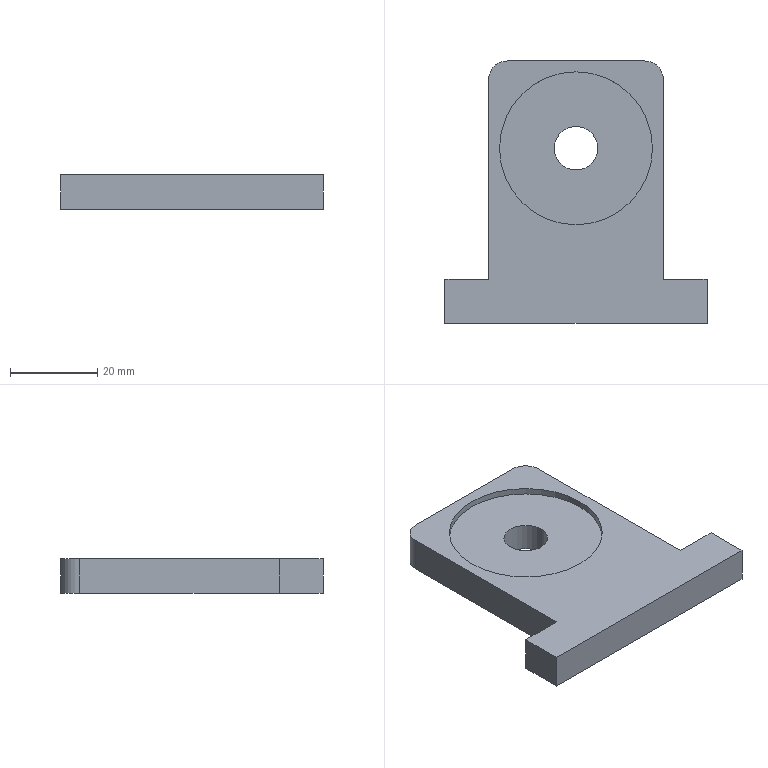Part | SolidWorks | 1 solid | 17 faces | box 60 x 60 x 8 mm | volume 18784 mm3 | plane 11 | cylinder 6 | commonest cylinder face diameters 8.5 x2 10 x2 35 x2
STEP:
#1=CARTESIAN_POINT('',(-5.,35.,0.));
#2=VERTEX_POINT('',#1);
#3=CARTESIAN_POINT('',(5.,35.,0.));
#4=VERTEX_POINT('',#3);
#5=CARTESIAN_POINT('',(0.,35.,0.));
#6=DIRECTION('',(0.,0.,1.));
#7=DIRECTION('',(1.,0.,0.));
#8=AXIS2_PLACEMENT_3D('',#5,#6,#7);
#9=CIRCLE('',#8,5.);
#10=EDGE_CURVE('',#2,#4,#9,.T.);
#11=ORIENTED_EDGE('',*,*,#10,.F.);
#12=CARTESIAN_POINT('',(-5.,35.,6.5));
#13=VERTEX_POINT('',#12);
#14=CARTESIAN_POINT('',(-5.,35.,-63.5));
#15=DIRECTION('',(0.,0.,1.));
#16=VECTOR('',#15,1000.);
#17=LINE('',#14,#16);
#18=EDGE_CURVE('',#2,#13,#17,.T.);
#19=ORIENTED_EDGE('',*,*,#18,.T.);
#20=CARTESIAN_POINT('',(5.,35.,6.5));
#21=VERTEX_POINT('',#20);
#22=CARTESIAN_POINT('',(0.,35.,6.5));
#23=DIRECTION('',(0.,0.,1.));
#24=DIRECTION('',(1.,0.,0.));
#25=AXIS2_PLACEMENT_3D('',#22,#23,#24);
#26=CIRCLE('',#25,5.);
#27=EDGE_CURVE('',#13,#21,#26,.T.);
#28=ORIENTED_EDGE('',*,*,#27,.T.);
#29=CARTESIAN_POINT('',(5.,35.,-63.5));
#30=DIRECTION('',(0.,0.,1.));
#31=VECTOR('',#30,1000.);
#32=LINE('',#29,#31);
#33=EDGE_CURVE('',#4,#21,#32,.T.);
#34=ORIENTED_EDGE('',*,*,#33,.F.);
#35=EDGE_LOOP('',(#11,#19,#28,#34));
#36=FACE_OUTER_BOUND('',#35,.T.);
#37=CARTESIAN_POINT('',(0.,35.,-63.5));
#38=DIRECTION('',(0.,0.,1.));
#39=DIRECTION('',(1.,0.,0.));
#40=AXIS2_PLACEMENT_3D('',#37,#38,#39);
#41=CYLINDRICAL_SURFACE('',#40,5.);
#42=ADVANCED_FACE('',(#36),#41,.F.);
#43=CARTESIAN_POINT('',(-17.5,35.,6.5));
#44=VERTEX_POINT('',#43);
#45=CARTESIAN_POINT('',(17.5,35.,6.5));
#46=VERTEX_POINT('',#45);
#47=CARTESIAN_POINT('',(0.,35.,6.5));
#48=DIRECTION('',(0.,0.,1.));
#49=DIRECTION('',(1.,0.,0.));
#50=AXIS2_PLACEMENT_3D('',#47,#48,#49);
#51=CIRCLE('',#50,17.5);
#52=EDGE_CURVE('',#44,#46,#51,.T.);
#53=ORIENTED_EDGE('',*,*,#52,.F.);
#54=CARTESIAN_POINT('',(-17.5,35.,8.));
#55=VERTEX_POINT('',#54);
#56=CARTESIAN_POINT('',(-17.5,35.,6.5));
#57=DIRECTION('',(0.,0.,1.));
#58=VECTOR('',#57,1000.);
#59=LINE('',#56,#58);
#60=EDGE_CURVE('',#44,#55,#59,.T.);
#61=ORIENTED_EDGE('',*,*,#60,.T.);
#62=CARTESIAN_POINT('',(17.5,35.,8.));
#63=VERTEX_POINT('',#62);
#64=CARTESIAN_POINT('',(0.,35.,8.));
#65=DIRECTION('',(0.,0.,1.));
#66=DIRECTION('',(1.,0.,0.));
#67=AXIS2_PLACEMENT_3D('',#64,#65,#66);
#68=CIRCLE('',#67,17.5);
#69=EDGE_CURVE('',#55,#63,#68,.T.);
#70=ORIENTED_EDGE('',*,*,#69,.T.);
#71=CARTESIAN_POINT('',(17.5,35.,6.5));
#72=DIRECTION('',(0.,0.,1.));
#73=VECTOR('',#72,1000.);
#74=LINE('',#71,#73);
#75=EDGE_CURVE('',#46,#63,#74,.T.);
#76=ORIENTED_EDGE('',*,*,#75,.F.);
#77=EDGE_LOOP('',(#53,#61,#70,#76));
#78=FACE_OUTER_BOUND('',#77,.T.);
#79=CARTESIAN_POINT('',(0.,35.,6.5));
#80=DIRECTION('',(0.,0.,1.));
#81=DIRECTION('',(1.,0.,0.));
#82=AXIS2_PLACEMENT_3D('',#79,#80,#81);
#83=CYLINDRICAL_SURFACE('',#82,17.5);
#84=ADVANCED_FACE('',(#78),#83,.F.);
#85=CARTESIAN_POINT('',(30.,-5.,0.));
#86=VERTEX_POINT('',#85);
#87=CARTESIAN_POINT('',(30.,5.,0.));
#88=VERTEX_POINT('',#87);
#89=CARTESIAN_POINT('',(30.,5.,0.));
#90=DIRECTION('',(0.,1.,0.));
#91=VECTOR('',#90,1000.);
#92=LINE('',#89,#91);
#93=EDGE_CURVE('',#86,#88,#92,.T.);
#94=ORIENTED_EDGE('',*,*,#93,.T.);
#95=CARTESIAN_POINT('',(30.,5.,8.));
#96=VERTEX_POINT('',#95);
#97=CARTESIAN_POINT('',(30.,5.,8.));
#98=DIRECTION('',(0.,0.,-1.));
#99=VECTOR('',#98,1000.);
#100=LINE('',#97,#99);
#101=EDGE_CURVE('',#96,#88,#100,.T.);
#102=ORIENTED_EDGE('',*,*,#101,.F.);
#103=CARTESIAN_POINT('',(30.,-5.,8.));
#104=VERTEX_POINT('',#103);
#105=CARTESIAN_POINT('',(30.,5.,8.));
#106=DIRECTION('',(0.,1.,0.));
#107=VECTOR('',#106,1000.);
#108=LINE('',#105,#107);
#109=EDGE_CURVE('',#104,#96,#108,.T.);
#110=ORIENTED_EDGE('',*,*,#109,.F.);
#111=CARTESIAN_POINT('',(30.,-5.,8.));
#112=DIRECTION('',(0.,0.,-1.));
#113=VECTOR('',#112,1000.);
#114=LINE('',#111,#113);
#115=EDGE_CURVE('',#104,#86,#114,.T.);
#116=ORIENTED_EDGE('',*,*,#115,.T.);
#117=EDGE_LOOP('',(#94,#102,#110,#116));
#118=FACE_OUTER_BOUND('',#117,.T.);
#119=CARTESIAN_POINT('',(30.,5.,8.));
#120=DIRECTION('',(-1.,0.,0.));
#121=DIRECTION('',(0.,0.,1.));
#122=AXIS2_PLACEMENT_3D('',#119,#120,#121);
#123=PLANE('',#122);
#124=ADVANCED_FACE('',(#118),#123,.F.);
#125=CARTESIAN_POINT('',(20.,5.,0.));
#126=VERTEX_POINT('',#125);
#127=CARTESIAN_POINT('',(20.,5.,0.));
#128=DIRECTION('',(-1.,0.,0.));
#129=VECTOR('',#128,1000.);
#130=LINE('',#127,#129);
#131=EDGE_CURVE('',#88,#126,#130,.T.);
#132=ORIENTED_EDGE('',*,*,#131,.T.);
#133=CARTESIAN_POINT('',(20.,5.,8.));
#134=VERTEX_POINT('',#133);
#135=CARTESIAN_POINT('',(20.,5.,8.));
#136=DIRECTION('',(0.,0.,-1.));
#137=VECTOR('',#136,1000.);
#138=LINE('',#135,#137);
#139=EDGE_CURVE('',#134,#126,#138,.T.);
#140=ORIENTED_EDGE('',*,*,#139,.F.);
#141=CARTESIAN_POINT('',(20.,5.,8.));
#142=DIRECTION('',(-1.,0.,0.));
#143=VECTOR('',#142,1000.);
#144=LINE('',#141,#143);
#145=EDGE_CURVE('',#96,#134,#144,.T.);
#146=ORIENTED_EDGE('',*,*,#145,.F.);
#147=ORIENTED_EDGE('',*,*,#101,.T.);
#148=EDGE_LOOP('',(#132,#140,#146,#147));
#149=FACE_OUTER_BOUND('',#148,.T.);
#150=CARTESIAN_POINT('',(20.,5.,8.));
#151=DIRECTION('',(0.,-1.,0.));
#152=DIRECTION('',(1.,0.,0.));
#153=AXIS2_PLACEMENT_3D('',#150,#151,#152);
#154=PLANE('',#153);
#155=ADVANCED_FACE('',(#149),#154,.F.);
#156=CARTESIAN_POINT('',(20.,50.75,0.));
#157=VERTEX_POINT('',#156);
#158=CARTESIAN_POINT('',(20.,5.,0.));
#159=DIRECTION('',(0.,1.,0.));
#160=VECTOR('',#159,1000.);
#161=LINE('',#158,#160);
#162=EDGE_CURVE('',#126,#157,#161,.T.);
#163=ORIENTED_EDGE('',*,*,#162,.T.);
#164=CARTESIAN_POINT('',(20.,50.75,8.));
#165=VERTEX_POINT('',#164);
#166=CARTESIAN_POINT('',(20.,50.75,8.));
#167=DIRECTION('',(0.,0.,1.));
#168=VECTOR('',#167,1000.);
#169=LINE('',#166,#168);
#170=EDGE_CURVE('',#157,#165,#169,.T.);
#171=ORIENTED_EDGE('',*,*,#170,.T.);
#172=CARTESIAN_POINT('',(20.,5.,8.));
#173=DIRECTION('',(0.,1.,0.));
#174=VECTOR('',#173,1000.);
#175=LINE('',#172,#174);
#176=EDGE_CURVE('',#134,#165,#175,.T.);
#177=ORIENTED_EDGE('',*,*,#176,.F.);
#178=ORIENTED_EDGE('',*,*,#139,.T.);
#179=EDGE_LOOP('',(#163,#171,#177,#178));
#180=FACE_OUTER_BOUND('',#179,.T.);
#181=CARTESIAN_POINT('',(20.,5.,8.));
#182=DIRECTION('',(-1.,0.,0.));
#183=DIRECTION('',(0.,-1.,0.));
#184=AXIS2_PLACEMENT_3D('',#181,#182,#183);
#185=PLANE('',#184);
#186=ADVANCED_FACE('',(#180),#185,.F.);
#187=CARTESIAN_POINT('',(15.75,55.,0.));
#188=VERTEX_POINT('',#187);
#189=CARTESIAN_POINT('',(-15.75,55.,0.));
#190=VERTEX_POINT('',#189);
#191=CARTESIAN_POINT('',(-20.,55.,0.));
#192=DIRECTION('',(-1.,0.,0.));
#193=VECTOR('',#192,1000.);
#194=LINE('',#191,#193);
#195=EDGE_CURVE('',#188,#190,#194,.T.);
#196=ORIENTED_EDGE('',*,*,#195,.T.);
#197=CARTESIAN_POINT('',(-15.75,55.,8.));
#198=VERTEX_POINT('',#197);
#199=CARTESIAN_POINT('',(-15.75,55.,8.));
#200=DIRECTION('',(0.,0.,1.));
#201=VECTOR('',#200,1000.);
#202=LINE('',#199,#201);
#203=EDGE_CURVE('',#190,#198,#202,.T.);
#204=ORIENTED_EDGE('',*,*,#203,.T.);
#205=CARTESIAN_POINT('',(15.75,55.,8.));
#206=VERTEX_POINT('',#205);
#207=CARTESIAN_POINT('',(-20.,55.,8.));
#208=DIRECTION('',(-1.,0.,0.));
#209=VECTOR('',#208,1000.);
#210=LINE('',#207,#209);
#211=EDGE_CURVE('',#206,#198,#210,.T.);
#212=ORIENTED_EDGE('',*,*,#211,.F.);
#213=CARTESIAN_POINT('',(15.75,55.,8.));
#214=DIRECTION('',(0.,0.,-1.));
#215=VECTOR('',#214,1000.);
#216=LINE('',#213,#215);
#217=EDGE_CURVE('',#206,#188,#216,.T.);
#218=ORIENTED_EDGE('',*,*,#217,.T.);
#219=EDGE_LOOP('',(#196,#204,#212,#218));
#220=FACE_OUTER_BOUND('',#219,.T.);
#221=CARTESIAN_POINT('',(-20.,55.,8.));
#222=DIRECTION('',(0.,-1.,0.));
#223=DIRECTION('',(1.,0.,0.));
#224=AXIS2_PLACEMENT_3D('',#221,#222,#223);
#225=PLANE('',#224);
#226=ADVANCED_FACE('',(#220),#225,.F.);
#227=CARTESIAN_POINT('',(-20.,50.75,8.));
#228=VERTEX_POINT('',#227);
#229=CARTESIAN_POINT('',(-20.,5.,8.));
#230=VERTEX_POINT('',#229);
#231=CARTESIAN_POINT('',(-20.,5.,8.));
#232=DIRECTION('',(0.,-1.,0.));
#233=VECTOR('',#232,1000.);
#234=LINE('',#231,#233);
#235=EDGE_CURVE('',#228,#230,#234,.T.);
#236=ORIENTED_EDGE('',*,*,#235,.F.);
#237=CARTESIAN_POINT('',(-20.,50.75,0.));
#238=VERTEX_POINT('',#237);
#239=CARTESIAN_POINT('',(-20.,50.75,8.));
#240=DIRECTION('',(0.,0.,-1.));
#241=VECTOR('',#240,1000.);
#242=LINE('',#239,#241);
#243=EDGE_CURVE('',#228,#238,#242,.T.);
#244=ORIENTED_EDGE('',*,*,#243,.T.);
#245=CARTESIAN_POINT('',(-20.,5.,0.));
#246=VERTEX_POINT('',#245);
#247=CARTESIAN_POINT('',(-20.,5.,0.));
#248=DIRECTION('',(0.,-1.,0.));
#249=VECTOR('',#248,1000.);
#250=LINE('',#247,#249);
#251=EDGE_CURVE('',#238,#246,#250,.T.);
#252=ORIENTED_EDGE('',*,*,#251,.T.);
#253=CARTESIAN_POINT('',(-20.,5.,8.));
#254=DIRECTION('',(0.,0.,-1.));
#255=VECTOR('',#254,1000.);
#256=LINE('',#253,#255);
#257=EDGE_CURVE('',#230,#246,#256,.T.);
#258=ORIENTED_EDGE('',*,*,#257,.F.);
#259=EDGE_LOOP('',(#236,#244,#252,#258));
#260=FACE_OUTER_BOUND('',#259,.T.);
#261=CARTESIAN_POINT('',(-20.,5.,8.));
#262=DIRECTION('',(1.,0.,0.));
#263=DIRECTION('',(0.,1.,0.));
#264=AXIS2_PLACEMENT_3D('',#261,#262,#263);
#265=PLANE('',#264);
#266=ADVANCED_FACE('',(#260),#265,.F.);
#267=CARTESIAN_POINT('',(-30.,5.,0.));
#268=VERTEX_POINT('',#267);
#269=CARTESIAN_POINT('',(-30.,5.,0.));
#270=DIRECTION('',(-1.,0.,0.));
#271=VECTOR('',#270,1000.);
#272=LINE('',#269,#271);
#273=EDGE_CURVE('',#246,#268,#272,.T.);
#274=ORIENTED_EDGE('',*,*,#273,.T.);
#275=CARTESIAN_POINT('',(-30.,5.,8.));
#276=VERTEX_POINT('',#275);
#277=CARTESIAN_POINT('',(-30.,5.,8.));
#278=DIRECTION('',(0.,0.,-1.));
#279=VECTOR('',#278,1000.);
#280=LINE('',#277,#279);
#281=EDGE_CURVE('',#276,#268,#280,.T.);
#282=ORIENTED_EDGE('',*,*,#281,.F.);
#283=CARTESIAN_POINT('',(-30.,5.,8.));
#284=DIRECTION('',(-1.,0.,0.));
#285=VECTOR('',#284,1000.);
#286=LINE('',#283,#285);
#287=EDGE_CURVE('',#230,#276,#286,.T.);
#288=ORIENTED_EDGE('',*,*,#287,.F.);
#289=ORIENTED_EDGE('',*,*,#257,.T.);
#290=EDGE_LOOP('',(#274,#282,#288,#289));
#291=FACE_OUTER_BOUND('',#290,.T.);
#292=CARTESIAN_POINT('',(-30.,5.,8.));
#293=DIRECTION('',(0.,-1.,0.));
#294=DIRECTION('',(1.,0.,0.));
#295=AXIS2_PLACEMENT_3D('',#292,#293,#294);
#296=PLANE('',#295);
#297=ADVANCED_FACE('',(#291),#296,.F.);
#298=CARTESIAN_POINT('',(-30.,-5.,0.));
#299=VERTEX_POINT('',#298);
#300=CARTESIAN_POINT('',(-30.,5.,0.));
#301=DIRECTION('',(0.,-1.,0.));
#302=VECTOR('',#301,1000.);
#303=LINE('',#300,#302);
#304=EDGE_CURVE('',#268,#299,#303,.T.);
#305=ORIENTED_EDGE('',*,*,#304,.T.);
#306=CARTESIAN_POINT('',(-30.,-5.,8.));
#307=VERTEX_POINT('',#306);
#308=CARTESIAN_POINT('',(-30.,-5.,8.));
#309=DIRECTION('',(0.,0.,-1.));
#310=VECTOR('',#309,1000.);
#311=LINE('',#308,#310);
#312=EDGE_CURVE('',#307,#299,#311,.T.);
#313=ORIENTED_EDGE('',*,*,#312,.F.);
#314=CARTESIAN_POINT('',(-30.,5.,8.));
#315=DIRECTION('',(0.,-1.,0.));
#316=VECTOR('',#315,1000.);
#317=LINE('',#314,#316);
#318=EDGE_CURVE('',#276,#307,#317,.T.);
#319=ORIENTED_EDGE('',*,*,#318,.F.);
#320=ORIENTED_EDGE('',*,*,#281,.T.);
#321=EDGE_LOOP('',(#305,#313,#319,#320));
#322=FACE_OUTER_BOUND('',#321,.T.);
#323=CARTESIAN_POINT('',(-30.,5.,8.));
#324=DIRECTION('',(1.,0.,0.));
#325=DIRECTION('',(0.,0.,-1.));
#326=AXIS2_PLACEMENT_3D('',#323,#324,#325);
#327=PLANE('',#326);
#328=ADVANCED_FACE('',(#322),#327,.F.);
#329=CARTESIAN_POINT('',(-30.,-5.,0.));
#330=DIRECTION('',(1.,0.,0.));
#331=VECTOR('',#330,1000.);
#332=LINE('',#329,#331);
#333=EDGE_CURVE('',#299,#86,#332,.T.);
#334=ORIENTED_EDGE('',*,*,#333,.T.);
#335=ORIENTED_EDGE('',*,*,#115,.F.);
#336=CARTESIAN_POINT('',(-30.,-5.,8.));
#337=DIRECTION('',(1.,0.,0.));
#338=VECTOR('',#337,1000.);
#339=LINE('',#336,#338);
#340=EDGE_CURVE('',#307,#104,#339,.T.);
#341=ORIENTED_EDGE('',*,*,#340,.F.);
#342=ORIENTED_EDGE('',*,*,#312,.T.);
#343=EDGE_LOOP('',(#334,#335,#341,#342));
#344=FACE_OUTER_BOUND('',#343,.T.);
#345=CARTESIAN_POINT('',(-30.,-5.,8.));
#346=DIRECTION('',(0.,1.,0.));
#347=DIRECTION('',(0.,0.,1.));
#348=AXIS2_PLACEMENT_3D('',#345,#346,#347);
#349=PLANE('',#348);
#350=ADVANCED_FACE('',(#344),#349,.F.);
#351=CARTESIAN_POINT('',(0.,35.,8.));
#352=DIRECTION('',(0.,0.,1.));
#353=DIRECTION('',(1.,0.,0.));
#354=AXIS2_PLACEMENT_3D('',#351,#352,#353);
#355=CIRCLE('',#354,17.5);
#356=EDGE_CURVE('',#63,#55,#355,.T.);
#357=ORIENTED_EDGE('',*,*,#356,.F.);
#358=ORIENTED_EDGE('',*,*,#69,.F.);
#359=EDGE_LOOP('',(#357,#358));
#360=FACE_BOUND('',#359,.T.);
#361=ORIENTED_EDGE('',*,*,#211,.T.);
#362=CARTESIAN_POINT('',(-15.75,50.75,8.));
#363=DIRECTION('',(0.,0.,1.));
#364=DIRECTION('',(1.,0.,0.));
#365=AXIS2_PLACEMENT_3D('',#362,#363,#364);
#366=CIRCLE('',#365,4.25);
#367=EDGE_CURVE('',#198,#228,#366,.T.);
#368=ORIENTED_EDGE('',*,*,#367,.T.);
#369=ORIENTED_EDGE('',*,*,#235,.T.);
#370=ORIENTED_EDGE('',*,*,#287,.T.);
#371=ORIENTED_EDGE('',*,*,#318,.T.);
#372=ORIENTED_EDGE('',*,*,#340,.T.);
#373=ORIENTED_EDGE('',*,*,#109,.T.);
#374=ORIENTED_EDGE('',*,*,#145,.T.);
#375=ORIENTED_EDGE('',*,*,#176,.T.);
#376=CARTESIAN_POINT('',(15.75,50.75,8.));
#377=DIRECTION('',(0.,0.,1.));
#378=DIRECTION('',(1.,0.,0.));
#379=AXIS2_PLACEMENT_3D('',#376,#377,#378);
#380=CIRCLE('',#379,4.25);
#381=EDGE_CURVE('',#165,#206,#380,.T.);
#382=ORIENTED_EDGE('',*,*,#381,.T.);
#383=EDGE_LOOP('',(#361,#368,#369,#370,#371,#372,#373,#374,#375,#382));
#384=FACE_OUTER_BOUND('',#383,.T.);
#385=CARTESIAN_POINT('',(0.,0.,8.));
#386=DIRECTION('',(0.,0.,1.));
#387=DIRECTION('',(1.,0.,0.));
#388=AXIS2_PLACEMENT_3D('',#385,#386,#387);
#389=PLANE('',#388);
#390=ADVANCED_FACE('',(#360,#384),#389,.T.);
#391=CARTESIAN_POINT('',(0.,35.,0.));
#392=DIRECTION('',(0.,0.,1.));
#393=DIRECTION('',(1.,0.,0.));
#394=AXIS2_PLACEMENT_3D('',#391,#392,#393);
#395=CIRCLE('',#394,5.);
#396=EDGE_CURVE('',#4,#2,#395,.T.);
#397=ORIENTED_EDGE('',*,*,#396,.T.);
#398=ORIENTED_EDGE('',*,*,#10,.T.);
#399=EDGE_LOOP('',(#397,#398));
#400=FACE_BOUND('',#399,.T.);
#401=ORIENTED_EDGE('',*,*,#251,.F.);
#402=CARTESIAN_POINT('',(-15.75,50.75,0.));
#403=DIRECTION('',(0.,0.,-1.));
#404=DIRECTION('',(1.,0.,0.));
#405=AXIS2_PLACEMENT_3D('',#402,#403,#404);
#406=CIRCLE('',#405,4.25);
#407=EDGE_CURVE('',#238,#190,#406,.T.);
#408=ORIENTED_EDGE('',*,*,#407,.T.);
#409=ORIENTED_EDGE('',*,*,#195,.F.);
#410=CARTESIAN_POINT('',(15.75,50.75,0.));
#411=DIRECTION('',(0.,0.,-1.));
#412=DIRECTION('',(1.,0.,0.));
#413=AXIS2_PLACEMENT_3D('',#410,#411,#412);
#414=CIRCLE('',#413,4.25);
#415=EDGE_CURVE('',#188,#157,#414,.T.);
#416=ORIENTED_EDGE('',*,*,#415,.T.);
#417=ORIENTED_EDGE('',*,*,#162,.F.);
#418=ORIENTED_EDGE('',*,*,#131,.F.);
#419=ORIENTED_EDGE('',*,*,#93,.F.);
#420=ORIENTED_EDGE('',*,*,#333,.F.);
#421=ORIENTED_EDGE('',*,*,#304,.F.);
#422=ORIENTED_EDGE('',*,*,#273,.F.);
#423=EDGE_LOOP('',(#401,#408,#409,#416,#417,#418,#419,#420,#421,#422));
#424=FACE_OUTER_BOUND('',#423,.T.);
#425=CARTESIAN_POINT('',(0.,0.,0.));
#426=DIRECTION('',(0.,0.,1.));
#427=DIRECTION('',(1.,0.,0.));
#428=AXIS2_PLACEMENT_3D('',#425,#426,#427);
#429=PLANE('',#428);
#430=ADVANCED_FACE('',(#400,#424),#429,.F.);
#431=ORIENTED_EDGE('',*,*,#60,.F.);
#432=CARTESIAN_POINT('',(0.,35.,6.5));
#433=DIRECTION('',(0.,0.,1.));
#434=DIRECTION('',(1.,0.,0.));
#435=AXIS2_PLACEMENT_3D('',#432,#433,#434);
#436=CIRCLE('',#435,17.5);
#437=EDGE_CURVE('',#46,#44,#436,.T.);
#438=ORIENTED_EDGE('',*,*,#437,.F.);
#439=ORIENTED_EDGE('',*,*,#75,.T.);
#440=ORIENTED_EDGE('',*,*,#356,.T.);
#441=EDGE_LOOP('',(#431,#438,#439,#440));
#442=FACE_OUTER_BOUND('',#441,.T.);
#443=CARTESIAN_POINT('',(0.,35.,6.5));
#444=DIRECTION('',(0.,0.,1.));
#445=DIRECTION('',(1.,0.,0.));
#446=AXIS2_PLACEMENT_3D('',#443,#444,#445);
#447=CYLINDRICAL_SURFACE('',#446,17.5);
#448=ADVANCED_FACE('',(#442),#447,.F.);
#449=CARTESIAN_POINT('',(0.,35.,6.5));
#450=DIRECTION('',(0.,0.,1.));
#451=DIRECTION('',(1.,0.,0.));
#452=AXIS2_PLACEMENT_3D('',#449,#450,#451);
#453=CIRCLE('',#452,5.);
#454=EDGE_CURVE('',#21,#13,#453,.T.);
#455=ORIENTED_EDGE('',*,*,#454,.F.);
#456=ORIENTED_EDGE('',*,*,#27,.F.);
#457=EDGE_LOOP('',(#455,#456));
#458=FACE_BOUND('',#457,.T.);
#459=ORIENTED_EDGE('',*,*,#437,.T.);
#460=ORIENTED_EDGE('',*,*,#52,.T.);
#461=EDGE_LOOP('',(#459,#460));
#462=FACE_OUTER_BOUND('',#461,.T.);
#463=CARTESIAN_POINT('',(0.,35.,6.5));
#464=DIRECTION('',(0.,0.,1.));
#465=DIRECTION('',(1.,0.,0.));
#466=AXIS2_PLACEMENT_3D('',#463,#464,#465);
#467=PLANE('',#466);
#468=ADVANCED_FACE('',(#458,#462),#467,.T.);
#469=ORIENTED_EDGE('',*,*,#18,.F.);
#470=ORIENTED_EDGE('',*,*,#396,.F.);
#471=ORIENTED_EDGE('',*,*,#33,.T.);
#472=ORIENTED_EDGE('',*,*,#454,.T.);
#473=EDGE_LOOP('',(#469,#470,#471,#472));
#474=FACE_OUTER_BOUND('',#473,.T.);
#475=CARTESIAN_POINT('',(0.,35.,-63.5));
#476=DIRECTION('',(0.,0.,1.));
#477=DIRECTION('',(1.,0.,0.));
#478=AXIS2_PLACEMENT_3D('',#475,#476,#477);
#479=CYLINDRICAL_SURFACE('',#478,5.);
#480=ADVANCED_FACE('',(#474),#479,.F.);
#481=ORIENTED_EDGE('',*,*,#367,.F.);
#482=ORIENTED_EDGE('',*,*,#203,.F.);
#483=ORIENTED_EDGE('',*,*,#407,.F.);
#484=ORIENTED_EDGE('',*,*,#243,.F.);
#485=EDGE_LOOP('',(#481,#482,#483,#484));
#486=FACE_OUTER_BOUND('',#485,.T.);
#487=CARTESIAN_POINT('',(-15.75,50.75,8.));
#488=DIRECTION('',(0.,0.,-1.));
#489=DIRECTION('',(-1.,0.,0.));
#490=AXIS2_PLACEMENT_3D('',#487,#488,#489);
#491=CYLINDRICAL_SURFACE('',#490,4.25);
#492=ADVANCED_FACE('',(#486),#491,.T.);
#493=ORIENTED_EDGE('',*,*,#381,.F.);
#494=ORIENTED_EDGE('',*,*,#170,.F.);
#495=ORIENTED_EDGE('',*,*,#415,.F.);
#496=ORIENTED_EDGE('',*,*,#217,.F.);
#497=EDGE_LOOP('',(#493,#494,#495,#496));
#498=FACE_OUTER_BOUND('',#497,.T.);
#499=CARTESIAN_POINT('',(15.75,50.75,8.));
#500=DIRECTION('',(0.,0.,-1.));
#501=DIRECTION('',(-1.,0.,0.));
#502=AXIS2_PLACEMENT_3D('',#499,#500,#501);
#503=CYLINDRICAL_SURFACE('',#502,4.25);
#504=ADVANCED_FACE('',(#498),#503,.T.);
#505=CLOSED_SHELL('',(#42,#84,#124,#155,#186,#226,#266,#297,#328,#350,#390,#430,#448,#468,#480,#492,#504));
#506=MANIFOLD_SOLID_BREP('',#505);
#507=CARTESIAN_POINT('',(0.,0.,0.));
#508=DIRECTION('',(0.,0.,1.));
#509=DIRECTION('',(1.,0.,0.));
#510=AXIS2_PLACEMENT_3D('',#507,#508,#509);
#511=(LENGTH_UNIT()NAMED_UNIT(*)SI_UNIT(.MILLI.,.METRE.));
#512=UNCERTAINTY_MEASURE_WITH_UNIT(LENGTH_MEASURE(0.00001),#511,'','');
#513=(NAMED_UNIT(*)PLANE_ANGLE_UNIT()SI_UNIT($,.RADIAN.));
#514=(NAMED_UNIT(*)SI_UNIT($,.STERADIAN.)SOLID_ANGLE_UNIT());
#515=(GEOMETRIC_REPRESENTATION_CONTEXT(3)GLOBAL_UNCERTAINTY_ASSIGNED_CONTEXT((#512))GLOBAL_UNIT_ASSIGNED_CONTEXT((#511,#513,#514))REPRESENTATION_CONTEXT('',''));
#516=ADVANCED_BREP_SHAPE_REPRESENTATION('',(#506,#510),#515);